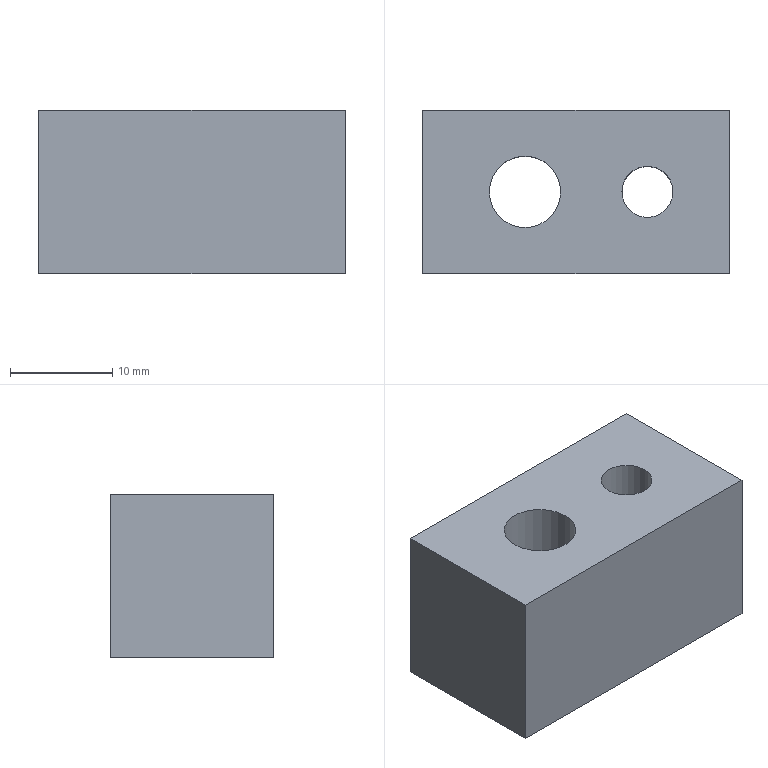Part | STEP file | gslz 2016.10.28-6_id262_x_t | 1 solid | 11 faces | box 30 x 16 x 16 mm | volume 6296 mm3 | plane 7 | cylinder 3 | cone 1 | commonest cylinder face diameters 5 x1 7 x1 11 x1
STEP:
#1=CARTESIAN_POINT('',(-67.95,150.,88.992));
#2=VERTEX_POINT('',#1);
#3=CARTESIAN_POINT('',(-70.95,150.,88.992));
#4=DIRECTION('',(0.,0.,-1.));
#5=DIRECTION('',(1.,0.,0.));
#6=AXIS2_PLACEMENT_3D('',#3,#4,#5);
#7=CIRCLE('',#6,3.);
#8=EDGE_CURVE('',#2,#2,#7,.T.);
#9=ORIENTED_EDGE('',*,*,#8,.F.);
#10=EDGE_LOOP('',(#9));
#11=FACE_BOUND('',#10,.T.);
#12=CARTESIAN_POINT('',(-92.95,158.,88.992));
#13=VERTEX_POINT('',#12);
#14=CARTESIAN_POINT('',(-92.95,142.,88.992));
#15=VERTEX_POINT('',#14);
#16=CARTESIAN_POINT('',(-92.95,158.,88.992));
#17=DIRECTION('',(0.,-1.,0.));
#18=VECTOR('',#17,1.);
#19=LINE('',#16,#18);
#20=EDGE_CURVE('',#13,#15,#19,.T.);
#21=ORIENTED_EDGE('',*,*,#20,.F.);
#22=CARTESIAN_POINT('',(-62.95,158.,88.992));
#23=VERTEX_POINT('',#22);
#24=CARTESIAN_POINT('',(-62.95,158.,88.992));
#25=DIRECTION('',(-1.,0.,0.));
#26=VECTOR('',#25,1.);
#27=LINE('',#24,#26);
#28=EDGE_CURVE('',#23,#13,#27,.T.);
#29=ORIENTED_EDGE('',*,*,#28,.F.);
#30=CARTESIAN_POINT('',(-62.95,142.,88.992));
#31=VERTEX_POINT('',#30);
#32=CARTESIAN_POINT('',(-62.95,142.,88.992));
#33=DIRECTION('',(0.,1.,0.));
#34=VECTOR('',#33,1.);
#35=LINE('',#32,#34);
#36=EDGE_CURVE('',#31,#23,#35,.T.);
#37=ORIENTED_EDGE('',*,*,#36,.F.);
#38=CARTESIAN_POINT('',(-92.95,142.,88.992));
#39=DIRECTION('',(1.,0.,0.));
#40=VECTOR('',#39,1.);
#41=LINE('',#38,#40);
#42=EDGE_CURVE('',#15,#31,#41,.T.);
#43=ORIENTED_EDGE('',*,*,#42,.F.);
#44=EDGE_LOOP('',(#21,#29,#37,#43));
#45=FACE_BOUND('',#44,.T.);
#46=CARTESIAN_POINT('',(-77.45,150.,88.992));
#47=VERTEX_POINT('',#46);
#48=CARTESIAN_POINT('',(-82.95,150.,88.992));
#49=DIRECTION('',(0.,0.,1.));
#50=DIRECTION('',(1.,0.,0.));
#51=AXIS2_PLACEMENT_3D('',#48,#49,#50);
#52=CIRCLE('',#51,5.5);
#53=EDGE_CURVE('',#47,#47,#52,.T.);
#54=ORIENTED_EDGE('',*,*,#53,.T.);
#55=EDGE_LOOP('',(#54));
#56=FACE_BOUND('',#55,.T.);
#57=CARTESIAN_POINT('',(-92.95,158.,88.992));
#58=DIRECTION('',(0.,0.,-1.));
#59=DIRECTION('',(-1.,0.,0.));
#60=AXIS2_PLACEMENT_3D('',#57,#58,#59);
#61=PLANE('',#60);
#62=ADVANCED_FACE('',(#11,#45,#56),#61,.T.);
#63=CARTESIAN_POINT('',(-68.45,150.,89.492));
#64=VERTEX_POINT('',#63);
#65=CARTESIAN_POINT('',(-70.95,150.,89.492));
#66=DIRECTION('',(0.,0.,1.));
#67=DIRECTION('',(1.,0.,0.));
#68=AXIS2_PLACEMENT_3D('',#65,#66,#67);
#69=CIRCLE('',#68,2.5);
#70=EDGE_CURVE('',#64,#64,#69,.T.);
#71=ORIENTED_EDGE('',*,*,#70,.F.);
#72=EDGE_LOOP('',(#71));
#73=FACE_BOUND('',#72,.T.);
#74=CARTESIAN_POINT('',(-68.45,150.,104.992));
#75=VERTEX_POINT('',#74);
#76=CARTESIAN_POINT('',(-70.95,150.,104.992));
#77=DIRECTION('',(0.,0.,-1.));
#78=DIRECTION('',(1.,0.,0.));
#79=AXIS2_PLACEMENT_3D('',#76,#77,#78);
#80=CIRCLE('',#79,2.5);
#81=EDGE_CURVE('',#75,#75,#80,.T.);
#82=ORIENTED_EDGE('',*,*,#81,.F.);
#83=EDGE_LOOP('',(#82));
#84=FACE_BOUND('',#83,.T.);
#85=CARTESIAN_POINT('',(-70.95,150.,72.992));
#86=DIRECTION('',(0.,0.,1.));
#87=DIRECTION('',(1.,0.,0.));
#88=AXIS2_PLACEMENT_3D('',#85,#86,#87);
#89=CYLINDRICAL_SURFACE('',#88,2.5);
#90=ADVANCED_FACE('',(#73,#84),#89,.F.);
#91=CARTESIAN_POINT('',(-79.45,150.,104.992));
#92=VERTEX_POINT('',#91);
#93=CARTESIAN_POINT('',(-82.95,150.,104.992));
#94=DIRECTION('',(0.,0.,-1.));
#95=DIRECTION('',(1.,0.,0.));
#96=AXIS2_PLACEMENT_3D('',#93,#94,#95);
#97=CIRCLE('',#96,3.5);
#98=EDGE_CURVE('',#92,#92,#97,.T.);
#99=ORIENTED_EDGE('',*,*,#98,.F.);
#100=EDGE_LOOP('',(#99));
#101=FACE_BOUND('',#100,.T.);
#102=CARTESIAN_POINT('',(-79.45,150.,96.992));
#103=VERTEX_POINT('',#102);
#104=CARTESIAN_POINT('',(-82.95,150.,96.992));
#105=DIRECTION('',(0.,0.,1.));
#106=DIRECTION('',(1.,0.,0.));
#107=AXIS2_PLACEMENT_3D('',#104,#105,#106);
#108=CIRCLE('',#107,3.5);
#109=EDGE_CURVE('',#103,#103,#108,.T.);
#110=ORIENTED_EDGE('',*,*,#109,.F.);
#111=EDGE_LOOP('',(#110));
#112=FACE_BOUND('',#111,.T.);
#113=CARTESIAN_POINT('',(-82.95,150.,72.992));
#114=DIRECTION('',(0.,0.,1.));
#115=DIRECTION('',(1.,0.,0.));
#116=AXIS2_PLACEMENT_3D('',#113,#114,#115);
#117=CYLINDRICAL_SURFACE('',#116,3.5);
#118=ADVANCED_FACE('',(#101,#112),#117,.F.);
#119=ORIENTED_EDGE('',*,*,#81,.T.);
#120=EDGE_LOOP('',(#119));
#121=FACE_BOUND('',#120,.T.);
#122=CARTESIAN_POINT('',(-92.95,142.,104.992));
#123=VERTEX_POINT('',#122);
#124=CARTESIAN_POINT('',(-62.95,142.,104.992));
#125=VERTEX_POINT('',#124);
#126=CARTESIAN_POINT('',(-92.95,142.,104.992));
#127=DIRECTION('',(1.,0.,0.));
#128=VECTOR('',#127,1.);
#129=LINE('',#126,#128);
#130=EDGE_CURVE('',#123,#125,#129,.T.);
#131=ORIENTED_EDGE('',*,*,#130,.T.);
#132=CARTESIAN_POINT('',(-62.95,158.,104.992));
#133=VERTEX_POINT('',#132);
#134=CARTESIAN_POINT('',(-62.95,142.,104.992));
#135=DIRECTION('',(0.,1.,0.));
#136=VECTOR('',#135,1.);
#137=LINE('',#134,#136);
#138=EDGE_CURVE('',#125,#133,#137,.T.);
#139=ORIENTED_EDGE('',*,*,#138,.T.);
#140=CARTESIAN_POINT('',(-92.95,158.,104.992));
#141=VERTEX_POINT('',#140);
#142=CARTESIAN_POINT('',(-62.95,158.,104.992));
#143=DIRECTION('',(-1.,0.,0.));
#144=VECTOR('',#143,1.);
#145=LINE('',#142,#144);
#146=EDGE_CURVE('',#133,#141,#145,.T.);
#147=ORIENTED_EDGE('',*,*,#146,.T.);
#148=CARTESIAN_POINT('',(-92.95,158.,104.992));
#149=DIRECTION('',(0.,-1.,0.));
#150=VECTOR('',#149,1.);
#151=LINE('',#148,#150);
#152=EDGE_CURVE('',#141,#123,#151,.T.);
#153=ORIENTED_EDGE('',*,*,#152,.T.);
#154=EDGE_LOOP('',(#131,#139,#147,#153));
#155=FACE_BOUND('',#154,.T.);
#156=ORIENTED_EDGE('',*,*,#98,.T.);
#157=EDGE_LOOP('',(#156));
#158=FACE_BOUND('',#157,.T.);
#159=CARTESIAN_POINT('',(-92.95,158.,104.992));
#160=DIRECTION('',(0.,0.,-1.));
#161=DIRECTION('',(-1.,0.,0.));
#162=AXIS2_PLACEMENT_3D('',#159,#160,#161);
#163=PLANE('',#162);
#164=ADVANCED_FACE('',(#121,#155,#158),#163,.F.);
#165=ORIENTED_EDGE('',*,*,#28,.T.);
#166=CARTESIAN_POINT('',(-92.95,158.,88.992));
#167=DIRECTION('',(0.,0.,1.));
#168=VECTOR('',#167,1.);
#169=LINE('',#166,#168);
#170=EDGE_CURVE('',#13,#141,#169,.T.);
#171=ORIENTED_EDGE('',*,*,#170,.T.);
#172=ORIENTED_EDGE('',*,*,#146,.F.);
#173=CARTESIAN_POINT('',(-62.95,158.,88.992));
#174=DIRECTION('',(0.,0.,1.));
#175=VECTOR('',#174,1.);
#176=LINE('',#173,#175);
#177=EDGE_CURVE('',#23,#133,#176,.T.);
#178=ORIENTED_EDGE('',*,*,#177,.F.);
#179=EDGE_LOOP('',(#165,#171,#172,#178));
#180=FACE_OUTER_BOUND('',#179,.T.);
#181=CARTESIAN_POINT('',(-62.95,158.,88.992));
#182=DIRECTION('',(0.,-1.,0.));
#183=DIRECTION('',(0.,0.,-1.));
#184=AXIS2_PLACEMENT_3D('',#181,#182,#183);
#185=PLANE('',#184);
#186=ADVANCED_FACE('',(#180),#185,.F.);
#187=ORIENTED_EDGE('',*,*,#152,.F.);
#188=ORIENTED_EDGE('',*,*,#170,.F.);
#189=ORIENTED_EDGE('',*,*,#20,.T.);
#190=CARTESIAN_POINT('',(-92.95,142.,88.992));
#191=DIRECTION('',(0.,0.,1.));
#192=VECTOR('',#191,1.);
#193=LINE('',#190,#192);
#194=EDGE_CURVE('',#15,#123,#193,.T.);
#195=ORIENTED_EDGE('',*,*,#194,.T.);
#196=EDGE_LOOP('',(#187,#188,#189,#195));
#197=FACE_OUTER_BOUND('',#196,.T.);
#198=CARTESIAN_POINT('',(-92.95,158.,88.992));
#199=DIRECTION('',(1.,0.,0.));
#200=DIRECTION('',(0.,0.,-1.));
#201=AXIS2_PLACEMENT_3D('',#198,#199,#200);
#202=PLANE('',#201);
#203=ADVANCED_FACE('',(#197),#202,.F.);
#204=ORIENTED_EDGE('',*,*,#42,.T.);
#205=CARTESIAN_POINT('',(-62.95,142.,88.992));
#206=DIRECTION('',(0.,0.,1.));
#207=VECTOR('',#206,1.);
#208=LINE('',#205,#207);
#209=EDGE_CURVE('',#31,#125,#208,.T.);
#210=ORIENTED_EDGE('',*,*,#209,.T.);
#211=ORIENTED_EDGE('',*,*,#130,.F.);
#212=ORIENTED_EDGE('',*,*,#194,.F.);
#213=EDGE_LOOP('',(#204,#210,#211,#212));
#214=FACE_OUTER_BOUND('',#213,.T.);
#215=CARTESIAN_POINT('',(-92.95,142.,88.992));
#216=DIRECTION('',(0.,1.,0.));
#217=DIRECTION('',(0.,0.,1.));
#218=AXIS2_PLACEMENT_3D('',#215,#216,#217);
#219=PLANE('',#218);
#220=ADVANCED_FACE('',(#214),#219,.F.);
#221=ORIENTED_EDGE('',*,*,#36,.T.);
#222=ORIENTED_EDGE('',*,*,#177,.T.);
#223=ORIENTED_EDGE('',*,*,#138,.F.);
#224=ORIENTED_EDGE('',*,*,#209,.F.);
#225=EDGE_LOOP('',(#221,#222,#223,#224));
#226=FACE_OUTER_BOUND('',#225,.T.);
#227=CARTESIAN_POINT('',(-62.95,142.,88.992));
#228=DIRECTION('',(-1.,0.,0.));
#229=DIRECTION('',(0.,0.,1.));
#230=AXIS2_PLACEMENT_3D('',#227,#228,#229);
#231=PLANE('',#230);
#232=ADVANCED_FACE('',(#226),#231,.F.);
#233=CARTESIAN_POINT('',(-77.45,150.,96.992));
#234=VERTEX_POINT('',#233);
#235=CARTESIAN_POINT('',(-82.95,150.,96.992));
#236=DIRECTION('',(0.,0.,-1.));
#237=DIRECTION('',(1.,0.,0.));
#238=AXIS2_PLACEMENT_3D('',#235,#236,#237);
#239=CIRCLE('',#238,5.5);
#240=EDGE_CURVE('',#234,#234,#239,.T.);
#241=ORIENTED_EDGE('',*,*,#240,.F.);
#242=EDGE_LOOP('',(#241));
#243=FACE_BOUND('',#242,.T.);
#244=ORIENTED_EDGE('',*,*,#53,.F.);
#245=EDGE_LOOP('',(#244));
#246=FACE_BOUND('',#245,.T.);
#247=CARTESIAN_POINT('',(-82.95,150.,96.992));
#248=DIRECTION('',(0.,0.,-1.));
#249=DIRECTION('',(-1.,0.,0.));
#250=AXIS2_PLACEMENT_3D('',#247,#248,#249);
#251=CYLINDRICAL_SURFACE('',#250,5.5);
#252=ADVANCED_FACE('',(#243,#246),#251,.F.);
#253=ORIENTED_EDGE('',*,*,#109,.T.);
#254=EDGE_LOOP('',(#253));
#255=FACE_BOUND('',#254,.T.);
#256=ORIENTED_EDGE('',*,*,#240,.T.);
#257=EDGE_LOOP('',(#256));
#258=FACE_BOUND('',#257,.T.);
#259=CARTESIAN_POINT('',(-82.95,150.,96.992));
#260=DIRECTION('',(0.,0.,-1.));
#261=DIRECTION('',(-1.,0.,0.));
#262=AXIS2_PLACEMENT_3D('',#259,#260,#261);
#263=PLANE('',#262);
#264=ADVANCED_FACE('',(#255,#258),#263,.T.);
#265=ORIENTED_EDGE('',*,*,#70,.T.);
#266=EDGE_LOOP('',(#265));
#267=FACE_BOUND('',#266,.T.);
#268=ORIENTED_EDGE('',*,*,#8,.T.);
#269=EDGE_LOOP('',(#268));
#270=FACE_BOUND('',#269,.T.);
#271=CARTESIAN_POINT('',(-70.95,150.,88.992));
#272=DIRECTION('',(0.,0.,-1.));
#273=DIRECTION('',(1.,0.,0.));
#274=AXIS2_PLACEMENT_3D('',#271,#272,#273);
#275=CONICAL_SURFACE('',#274,3.,45.);
#276=ADVANCED_FACE('',(#267,#270),#275,.F.);
#277=CLOSED_SHELL('',(#62,#90,#118,#164,#186,#203,#220,#232,#252,#264,#276));
#278=MANIFOLD_SOLID_BREP('',#277);
#279=(LENGTH_UNIT()NAMED_UNIT(*)SI_UNIT(.MILLI.,.METRE.));
#280=UNCERTAINTY_MEASURE_WITH_UNIT(LENGTH_MEASURE(0.00002),#279,'','');
#281=(NAMED_UNIT(*)PLANE_ANGLE_UNIT()SI_UNIT($,.RADIAN.));
#282=PLANE_ANGLE_MEASURE_WITH_UNIT(PLANE_ANGLE_MEASURE(0.01745),#281);
#283=DIMENSIONAL_EXPONENTS(0.,0.,0.,0.,0.,0.,0.);
#284=(CONVERSION_BASED_UNIT('DEGREE',#282)NAMED_UNIT(#283)PLANE_ANGLE_UNIT());
#285=(NAMED_UNIT(*)SI_UNIT($,.STERADIAN.)SOLID_ANGLE_UNIT());
#286=(GEOMETRIC_REPRESENTATION_CONTEXT(3)GLOBAL_UNCERTAINTY_ASSIGNED_CONTEXT((#280))GLOBAL_UNIT_ASSIGNED_CONTEXT((#279,#284,#285))REPRESENTATION_CONTEXT('',''));
#287=ADVANCED_BREP_SHAPE_REPRESENTATION('',(#278),#286);